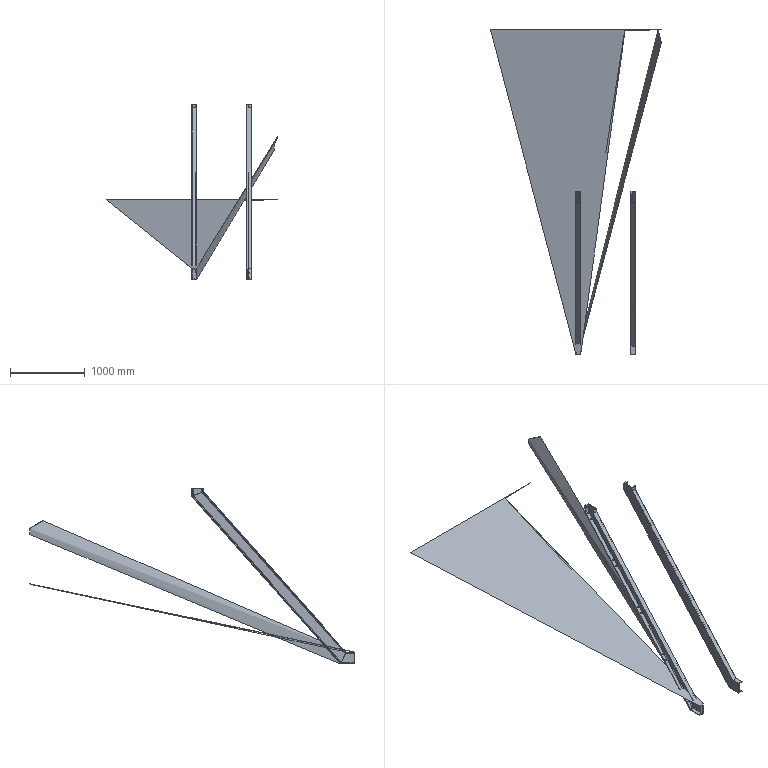Part | STEP file | 中转釜楼梯主体_Default<As Machined> | 6 solids | 126 faces | box 2295 x 4350 x 2360 mm | volume 95439230 mm3 | cylinder 66 | plane 60 | commonest cylinder face diameters 12 x40 10 x12 20 x12 13 x2